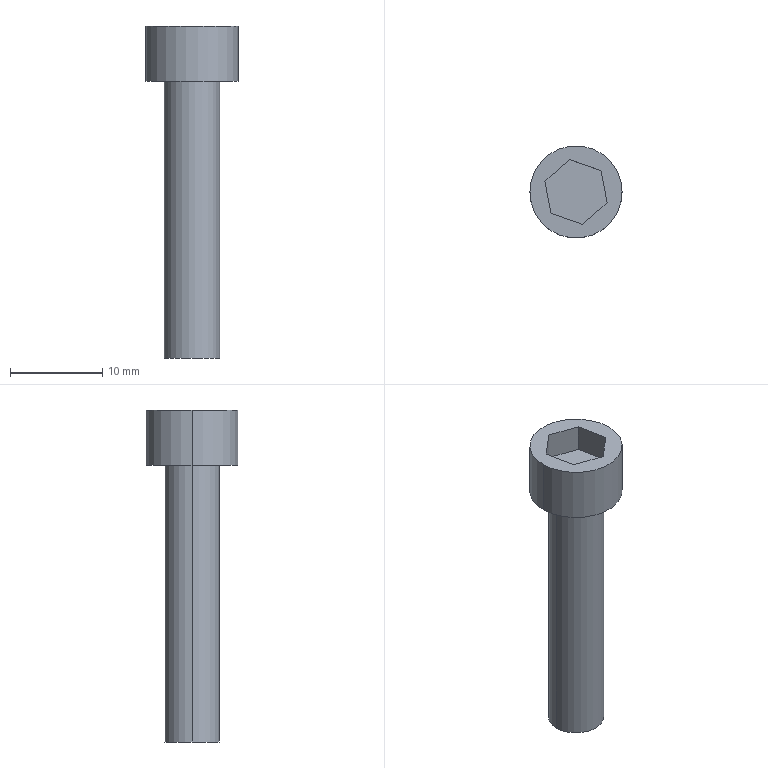Part | STEP file | M6 | 1 solid | 14 faces | box 10 x 10 x 36 mm | volume 1220 mm3 | plane 10 | cylinder 4 | commonest cylinder face diameters 6 x2 10 x2
STEP:
#1=CARTESIAN_POINT('',(0.,0.,0.));
#2=DIRECTION('',(0.,0.,1.));
#3=DIRECTION('',(1.,0.,0.));
#4=AXIS2_PLACEMENT_3D('',#1,#2,#3);
#5=CARTESIAN_POINT('',(-3.,0.,-30.));
#6=VERTEX_POINT('',#5);
#7=CARTESIAN_POINT('',(3.,0.,-30.));
#8=VERTEX_POINT('',#7);
#9=CARTESIAN_POINT('',(0.,0.,-30.));
#10=DIRECTION('',(0.,0.,-1.));
#11=DIRECTION('',(-1.,0.,0.));
#12=AXIS2_PLACEMENT_3D('',#9,#10,#11);
#13=CIRCLE('',#12,3.);
#14=CARTESIAN_POINT('',(0.,0.,-30.));
#15=DIRECTION('',(0.,0.,1.));
#16=DIRECTION('',(1.,0.,0.));
#17=AXIS2_PLACEMENT_3D('',#14,#15,#16);
#18=CYLINDRICAL_SURFACE('',#17,3.);
#19=CARTESIAN_POINT('',(3.142,0.));
#20=DIRECTION('',(-1.,0.));
#21=VECTOR('',#20,1.);
#22=LINE('',#19,#21);
#23=(GEOMETRIC_REPRESENTATION_CONTEXT(2)PARAMETRIC_REPRESENTATION_CONTEXT()REPRESENTATION_CONTEXT('',''));
#24=DEFINITIONAL_REPRESENTATION('',(#22),#23);
#25=PCURVE('',#18,#24);
#26=CARTESIAN_POINT('',(0.,0.,-30.));
#27=DIRECTION('',(0.,0.,-1.));
#28=DIRECTION('',(-1.,0.,0.));
#29=AXIS2_PLACEMENT_3D('',#26,#27,#28);
#30=PLANE('',#29);
#31=CARTESIAN_POINT('',(0.,0.));
#32=DIRECTION('',(1.,0.));
#33=AXIS2_PLACEMENT_2D('',#31,#32);
#34=CIRCLE('',#33,3.);
#35=(GEOMETRIC_REPRESENTATION_CONTEXT(2)PARAMETRIC_REPRESENTATION_CONTEXT()REPRESENTATION_CONTEXT('',''));
#36=DEFINITIONAL_REPRESENTATION('',(#34),#35);
#37=PCURVE('',#30,#36);
#38=SURFACE_CURVE('',#13,(#25,#37),.PCURVE_S1.);
#39=EDGE_CURVE('',#6,#8,#38,.T.);
#40=ORIENTED_EDGE('',*,*,#39,.F.);
#41=CARTESIAN_POINT('',(-3.,0.,0.));
#42=VERTEX_POINT('',#41);
#43=CARTESIAN_POINT('',(-3.,0.,-30.));
#44=DIRECTION('',(0.,0.,1.));
#45=VECTOR('',#44,1.);
#46=LINE('',#43,#45);
#47=CARTESIAN_POINT('',(3.142,0.));
#48=DIRECTION('',(0.,1.));
#49=VECTOR('',#48,1.);
#50=LINE('',#47,#49);
#51=(GEOMETRIC_REPRESENTATION_CONTEXT(2)PARAMETRIC_REPRESENTATION_CONTEXT()REPRESENTATION_CONTEXT('',''));
#52=DEFINITIONAL_REPRESENTATION('',(#50),#51);
#53=PCURVE('',#18,#52);
#54=CARTESIAN_POINT('',(0.,0.,-30.));
#55=DIRECTION('',(0.,0.,1.));
#56=DIRECTION('',(1.,0.,0.));
#57=AXIS2_PLACEMENT_3D('',#54,#55,#56);
#58=CYLINDRICAL_SURFACE('',#57,3.);
#59=CARTESIAN_POINT('',(3.142,0.));
#60=DIRECTION('',(0.,1.));
#61=VECTOR('',#60,1.);
#62=LINE('',#59,#61);
#63=(GEOMETRIC_REPRESENTATION_CONTEXT(2)PARAMETRIC_REPRESENTATION_CONTEXT()REPRESENTATION_CONTEXT('',''));
#64=DEFINITIONAL_REPRESENTATION('',(#62),#63);
#65=PCURVE('',#58,#64);
#66=SURFACE_CURVE('',#46,(#53,#65),.PCURVE_S1.);
#67=EDGE_CURVE('',#6,#42,#66,.T.);
#68=ORIENTED_EDGE('',*,*,#67,.T.);
#69=CARTESIAN_POINT('',(3.,0.,0.));
#70=VERTEX_POINT('',#69);
#71=CARTESIAN_POINT('',(0.,0.,0.));
#72=DIRECTION('',(0.,0.,-1.));
#73=DIRECTION('',(1.,0.,0.));
#74=AXIS2_PLACEMENT_3D('',#71,#72,#73);
#75=CIRCLE('',#74,3.);
#76=CARTESIAN_POINT('',(6.283,30.));
#77=DIRECTION('',(-1.,0.));
#78=VECTOR('',#77,1.);
#79=LINE('',#76,#78);
#80=(GEOMETRIC_REPRESENTATION_CONTEXT(2)PARAMETRIC_REPRESENTATION_CONTEXT()REPRESENTATION_CONTEXT('',''));
#81=DEFINITIONAL_REPRESENTATION('',(#79),#80);
#82=PCURVE('',#18,#81);
#83=CARTESIAN_POINT('',(0.,0.,0.));
#84=DIRECTION('',(0.,0.,1.));
#85=DIRECTION('',(1.,0.,0.));
#86=AXIS2_PLACEMENT_3D('',#83,#84,#85);
#87=PLANE('',#86);
#88=CARTESIAN_POINT('',(3.,0.));
#89=CARTESIAN_POINT('',(3.,-5.196));
#90=CARTESIAN_POINT('',(-1.5,-2.598));
#91=CARTESIAN_POINT('',(-6.,0.));
#92=CARTESIAN_POINT('',(-1.5,2.598));
#93=CARTESIAN_POINT('',(3.,5.196));
#94=CARTESIAN_POINT('',(3.,0.));
#95=(BOUNDED_CURVE()B_SPLINE_CURVE(2,(#88,#89,#90,#91,#92,#93,#94),.UNSPECIFIED.,.T.,.F.)B_SPLINE_CURVE_WITH_KNOTS((1,2,2,2,2,1),(-2.094,0.,2.094,4.189,6.283,8.378),.UNSPECIFIED.)CURVE()GEOMETRIC_REPRESENTATION_ITEM()RATIONAL_B_SPLINE_CURVE((1.,0.5,1.,0.5,1.,0.5,1.))REPRESENTATION_ITEM(''));
#96=(GEOMETRIC_REPRESENTATION_CONTEXT(2)PARAMETRIC_REPRESENTATION_CONTEXT()REPRESENTATION_CONTEXT('',''));
#97=DEFINITIONAL_REPRESENTATION('',(#95),#96);
#98=PCURVE('',#87,#97);
#99=SURFACE_CURVE('',#75,(#82,#98),.PCURVE_S1.);
#100=EDGE_CURVE('',#42,#70,#99,.T.);
#101=ORIENTED_EDGE('',*,*,#100,.T.);
#102=CARTESIAN_POINT('',(3.,0.,-30.));
#103=DIRECTION('',(0.,0.,1.));
#104=VECTOR('',#103,1.);
#105=LINE('',#102,#104);
#106=CARTESIAN_POINT('',(0.,0.));
#107=DIRECTION('',(0.,1.));
#108=VECTOR('',#107,1.);
#109=LINE('',#106,#108);
#110=(GEOMETRIC_REPRESENTATION_CONTEXT(2)PARAMETRIC_REPRESENTATION_CONTEXT()REPRESENTATION_CONTEXT('',''));
#111=DEFINITIONAL_REPRESENTATION('',(#109),#110);
#112=PCURVE('',#18,#111);
#113=CARTESIAN_POINT('',(6.283,0.));
#114=DIRECTION('',(0.,1.));
#115=VECTOR('',#114,1.);
#116=LINE('',#113,#115);
#117=(GEOMETRIC_REPRESENTATION_CONTEXT(2)PARAMETRIC_REPRESENTATION_CONTEXT()REPRESENTATION_CONTEXT('',''));
#118=DEFINITIONAL_REPRESENTATION('',(#116),#117);
#119=PCURVE('',#58,#118);
#120=SURFACE_CURVE('',#105,(#112,#119),.PCURVE_S1.);
#121=EDGE_CURVE('',#8,#70,#120,.T.);
#122=ORIENTED_EDGE('',*,*,#121,.F.);
#123=EDGE_LOOP('',(#40,#68,#101,#122));
#124=FACE_BOUND('',#123,.T.);
#125=ADVANCED_FACE('',(#124),#18,.T.);
#126=CARTESIAN_POINT('',(5.,0.,6.));
#127=VERTEX_POINT('',#126);
#128=CARTESIAN_POINT('',(-5.,0.,6.));
#129=VERTEX_POINT('',#128);
#130=CARTESIAN_POINT('',(0.,0.,6.));
#131=DIRECTION('',(0.,0.,1.));
#132=DIRECTION('',(1.,0.,0.));
#133=AXIS2_PLACEMENT_3D('',#130,#131,#132);
#134=CIRCLE('',#133,5.);
#135=CARTESIAN_POINT('',(0.,0.,6.));
#136=DIRECTION('',(0.,0.,-1.));
#137=DIRECTION('',(-1.,0.,0.));
#138=AXIS2_PLACEMENT_3D('',#135,#136,#137);
#139=CYLINDRICAL_SURFACE('',#138,5.);
#140=CARTESIAN_POINT('',(3.142,0.));
#141=DIRECTION('',(-1.,0.));
#142=VECTOR('',#141,1.);
#143=LINE('',#140,#142);
#144=(GEOMETRIC_REPRESENTATION_CONTEXT(2)PARAMETRIC_REPRESENTATION_CONTEXT()REPRESENTATION_CONTEXT('',''));
#145=DEFINITIONAL_REPRESENTATION('',(#143),#144);
#146=PCURVE('',#139,#145);
#147=CARTESIAN_POINT('',(0.,0.,6.));
#148=DIRECTION('',(0.,0.,1.));
#149=DIRECTION('',(1.,0.,0.));
#150=AXIS2_PLACEMENT_3D('',#147,#148,#149);
#151=PLANE('',#150);
#152=CARTESIAN_POINT('',(0.,0.));
#153=DIRECTION('',(1.,0.));
#154=AXIS2_PLACEMENT_2D('',#152,#153);
#155=CIRCLE('',#154,5.);
#156=(GEOMETRIC_REPRESENTATION_CONTEXT(2)PARAMETRIC_REPRESENTATION_CONTEXT()REPRESENTATION_CONTEXT('',''));
#157=DEFINITIONAL_REPRESENTATION('',(#155),#156);
#158=PCURVE('',#151,#157);
#159=SURFACE_CURVE('',#134,(#146,#158),.PCURVE_S1.);
#160=EDGE_CURVE('',#127,#129,#159,.T.);
#161=ORIENTED_EDGE('',*,*,#160,.F.);
#162=CARTESIAN_POINT('',(5.,0.,0.));
#163=VERTEX_POINT('',#162);
#164=CARTESIAN_POINT('',(5.,0.,6.));
#165=DIRECTION('',(0.,0.,-1.));
#166=VECTOR('',#165,1.);
#167=LINE('',#164,#166);
#168=CARTESIAN_POINT('',(3.142,0.));
#169=DIRECTION('',(0.,1.));
#170=VECTOR('',#169,1.);
#171=LINE('',#168,#170);
#172=(GEOMETRIC_REPRESENTATION_CONTEXT(2)PARAMETRIC_REPRESENTATION_CONTEXT()REPRESENTATION_CONTEXT('',''));
#173=DEFINITIONAL_REPRESENTATION('',(#171),#172);
#174=PCURVE('',#139,#173);
#175=CARTESIAN_POINT('',(0.,0.,6.));
#176=DIRECTION('',(0.,0.,-1.));
#177=DIRECTION('',(-1.,0.,0.));
#178=AXIS2_PLACEMENT_3D('',#175,#176,#177);
#179=CYLINDRICAL_SURFACE('',#178,5.);
#180=CARTESIAN_POINT('',(3.142,0.));
#181=DIRECTION('',(0.,1.));
#182=VECTOR('',#181,1.);
#183=LINE('',#180,#182);
#184=(GEOMETRIC_REPRESENTATION_CONTEXT(2)PARAMETRIC_REPRESENTATION_CONTEXT()REPRESENTATION_CONTEXT('',''));
#185=DEFINITIONAL_REPRESENTATION('',(#183),#184);
#186=PCURVE('',#179,#185);
#187=SURFACE_CURVE('',#167,(#174,#186),.PCURVE_S1.);
#188=EDGE_CURVE('',#127,#163,#187,.T.);
#189=ORIENTED_EDGE('',*,*,#188,.T.);
#190=CARTESIAN_POINT('',(-5.,0.,0.));
#191=VERTEX_POINT('',#190);
#192=CARTESIAN_POINT('',(0.,0.,0.));
#193=DIRECTION('',(0.,0.,1.));
#194=DIRECTION('',(1.,0.,0.));
#195=AXIS2_PLACEMENT_3D('',#192,#193,#194);
#196=CIRCLE('',#195,5.);
#197=CARTESIAN_POINT('',(3.142,6.));
#198=DIRECTION('',(-1.,0.));
#199=VECTOR('',#198,1.);
#200=LINE('',#197,#199);
#201=(GEOMETRIC_REPRESENTATION_CONTEXT(2)PARAMETRIC_REPRESENTATION_CONTEXT()REPRESENTATION_CONTEXT('',''));
#202=DEFINITIONAL_REPRESENTATION('',(#200),#201);
#203=PCURVE('',#139,#202);
#204=CARTESIAN_POINT('',(0.,0.));
#205=DIRECTION('',(1.,0.));
#206=AXIS2_PLACEMENT_2D('',#204,#205);
#207=CIRCLE('',#206,5.);
#208=(GEOMETRIC_REPRESENTATION_CONTEXT(2)PARAMETRIC_REPRESENTATION_CONTEXT()REPRESENTATION_CONTEXT('',''));
#209=DEFINITIONAL_REPRESENTATION('',(#207),#208);
#210=PCURVE('',#87,#209);
#211=SURFACE_CURVE('',#196,(#203,#210),.PCURVE_S1.);
#212=EDGE_CURVE('',#163,#191,#211,.T.);
#213=ORIENTED_EDGE('',*,*,#212,.T.);
#214=CARTESIAN_POINT('',(-5.,0.,6.));
#215=DIRECTION('',(0.,0.,-1.));
#216=VECTOR('',#215,1.);
#217=LINE('',#214,#216);
#218=CARTESIAN_POINT('',(0.,0.));
#219=DIRECTION('',(0.,1.));
#220=VECTOR('',#219,1.);
#221=LINE('',#218,#220);
#222=(GEOMETRIC_REPRESENTATION_CONTEXT(2)PARAMETRIC_REPRESENTATION_CONTEXT()REPRESENTATION_CONTEXT('',''));
#223=DEFINITIONAL_REPRESENTATION('',(#221),#222);
#224=PCURVE('',#139,#223);
#225=CARTESIAN_POINT('',(6.283,0.));
#226=DIRECTION('',(0.,1.));
#227=VECTOR('',#226,1.);
#228=LINE('',#225,#227);
#229=(GEOMETRIC_REPRESENTATION_CONTEXT(2)PARAMETRIC_REPRESENTATION_CONTEXT()REPRESENTATION_CONTEXT('',''));
#230=DEFINITIONAL_REPRESENTATION('',(#228),#229);
#231=PCURVE('',#179,#230);
#232=SURFACE_CURVE('',#217,(#224,#231),.PCURVE_S1.);
#233=EDGE_CURVE('',#129,#191,#232,.T.);
#234=ORIENTED_EDGE('',*,*,#233,.F.);
#235=EDGE_LOOP('',(#161,#189,#213,#234));
#236=FACE_BOUND('',#235,.T.);
#237=ADVANCED_FACE('',(#236),#139,.T.);
#238=CARTESIAN_POINT('',(0.,0.,0.));
#239=DIRECTION('',(0.,0.,1.));
#240=DIRECTION('',(1.,0.,0.));
#241=AXIS2_PLACEMENT_3D('',#238,#239,#240);
#242=CIRCLE('',#241,5.);
#243=CARTESIAN_POINT('',(0.,0.));
#244=DIRECTION('',(1.,0.));
#245=AXIS2_PLACEMENT_2D('',#243,#244);
#246=CIRCLE('',#245,5.);
#247=(GEOMETRIC_REPRESENTATION_CONTEXT(2)PARAMETRIC_REPRESENTATION_CONTEXT()REPRESENTATION_CONTEXT('',''));
#248=DEFINITIONAL_REPRESENTATION('',(#246),#247);
#249=PCURVE('',#87,#248);
#250=CARTESIAN_POINT('',(9.425,6.));
#251=DIRECTION('',(-1.,0.));
#252=VECTOR('',#251,1.);
#253=LINE('',#250,#252);
#254=(GEOMETRIC_REPRESENTATION_CONTEXT(2)PARAMETRIC_REPRESENTATION_CONTEXT()REPRESENTATION_CONTEXT('',''));
#255=DEFINITIONAL_REPRESENTATION('',(#253),#254);
#256=PCURVE('',#179,#255);
#257=SURFACE_CURVE('',#242,(#249,#256),.PCURVE_S1.);
#258=EDGE_CURVE('',#191,#163,#257,.T.);
#259=ORIENTED_EDGE('',*,*,#258,.F.);
#260=ORIENTED_EDGE('',*,*,#212,.F.);
#261=EDGE_LOOP('',(#259,#260));
#262=FACE_BOUND('',#261,.T.);
#263=CARTESIAN_POINT('',(0.,0.,0.));
#264=DIRECTION('',(0.,0.,-1.));
#265=DIRECTION('',(1.,0.,0.));
#266=AXIS2_PLACEMENT_3D('',#263,#264,#265);
#267=CIRCLE('',#266,3.);
#268=CARTESIAN_POINT('',(3.,0.));
#269=CARTESIAN_POINT('',(3.,-5.196));
#270=CARTESIAN_POINT('',(-1.5,-2.598));
#271=CARTESIAN_POINT('',(-6.,0.));
#272=CARTESIAN_POINT('',(-1.5,2.598));
#273=CARTESIAN_POINT('',(3.,5.196));
#274=CARTESIAN_POINT('',(3.,0.));
#275=(BOUNDED_CURVE()B_SPLINE_CURVE(2,(#268,#269,#270,#271,#272,#273,#274),.UNSPECIFIED.,.T.,.F.)B_SPLINE_CURVE_WITH_KNOTS((1,2,2,2,2,1),(-2.094,0.,2.094,4.189,6.283,8.378),.UNSPECIFIED.)CURVE()GEOMETRIC_REPRESENTATION_ITEM()RATIONAL_B_SPLINE_CURVE((1.,0.5,1.,0.5,1.,0.5,1.))REPRESENTATION_ITEM(''));
#276=(GEOMETRIC_REPRESENTATION_CONTEXT(2)PARAMETRIC_REPRESENTATION_CONTEXT()REPRESENTATION_CONTEXT('',''));
#277=DEFINITIONAL_REPRESENTATION('',(#275),#276);
#278=PCURVE('',#87,#277);
#279=CARTESIAN_POINT('',(6.283,30.));
#280=DIRECTION('',(-1.,0.));
#281=VECTOR('',#280,1.);
#282=LINE('',#279,#281);
#283=(GEOMETRIC_REPRESENTATION_CONTEXT(2)PARAMETRIC_REPRESENTATION_CONTEXT()REPRESENTATION_CONTEXT('',''));
#284=DEFINITIONAL_REPRESENTATION('',(#282),#283);
#285=PCURVE('',#58,#284);
#286=SURFACE_CURVE('',#267,(#278,#285),.PCURVE_S1.);
#287=EDGE_CURVE('',#70,#42,#286,.T.);
#288=ORIENTED_EDGE('',*,*,#287,.F.);
#289=ORIENTED_EDGE('',*,*,#100,.F.);
#290=EDGE_LOOP('',(#288,#289));
#291=FACE_BOUND('',#290,.T.);
#292=ADVANCED_FACE('',(#262,#291),#87,.F.);
#293=ORIENTED_EDGE('',*,*,#188,.F.);
#294=CARTESIAN_POINT('',(0.,0.,6.));
#295=DIRECTION('',(0.,0.,1.));
#296=DIRECTION('',(1.,0.,0.));
#297=AXIS2_PLACEMENT_3D('',#294,#295,#296);
#298=CIRCLE('',#297,5.);
#299=CARTESIAN_POINT('',(9.425,0.));
#300=DIRECTION('',(-1.,0.));
#301=VECTOR('',#300,1.);
#302=LINE('',#299,#301);
#303=(GEOMETRIC_REPRESENTATION_CONTEXT(2)PARAMETRIC_REPRESENTATION_CONTEXT()REPRESENTATION_CONTEXT('',''));
#304=DEFINITIONAL_REPRESENTATION('',(#302),#303);
#305=PCURVE('',#179,#304);
#306=CARTESIAN_POINT('',(0.,0.));
#307=DIRECTION('',(1.,0.));
#308=AXIS2_PLACEMENT_2D('',#306,#307);
#309=CIRCLE('',#308,5.);
#310=(GEOMETRIC_REPRESENTATION_CONTEXT(2)PARAMETRIC_REPRESENTATION_CONTEXT()REPRESENTATION_CONTEXT('',''));
#311=DEFINITIONAL_REPRESENTATION('',(#309),#310);
#312=PCURVE('',#151,#311);
#313=SURFACE_CURVE('',#298,(#305,#312),.PCURVE_S1.);
#314=EDGE_CURVE('',#129,#127,#313,.T.);
#315=ORIENTED_EDGE('',*,*,#314,.F.);
#316=ORIENTED_EDGE('',*,*,#233,.T.);
#317=ORIENTED_EDGE('',*,*,#258,.T.);
#318=EDGE_LOOP('',(#293,#315,#316,#317));
#319=FACE_BOUND('',#318,.T.);
#320=ADVANCED_FACE('',(#319),#179,.T.);
#321=CARTESIAN_POINT('',(-3.378,1.179,6.));
#322=VERTEX_POINT('',#321);
#323=CARTESIAN_POINT('',(-2.71,-2.336,6.));
#324=VERTEX_POINT('',#323);
#325=CARTESIAN_POINT('',(-3.378,1.179,6.));
#326=DIRECTION('',(0.1867,-0.9824,0.));
#327=VECTOR('',#326,1.);
#328=LINE('',#325,#327);
#329=CARTESIAN_POINT('',(-3.378,1.179));
#330=DIRECTION('',(0.1867,-0.9824));
#331=VECTOR('',#330,1.);
#332=LINE('',#329,#331);
#333=(GEOMETRIC_REPRESENTATION_CONTEXT(2)PARAMETRIC_REPRESENTATION_CONTEXT()REPRESENTATION_CONTEXT('',''));
#334=DEFINITIONAL_REPRESENTATION('',(#332),#333);
#335=PCURVE('',#151,#334);
#336=CARTESIAN_POINT('',(-3.378,1.179,3.));
#337=DIRECTION('',(-0.9824,-0.1867,0.));
#338=DIRECTION('',(0.1867,-0.9824,0.));
#339=AXIS2_PLACEMENT_3D('',#336,#337,#338);
#340=PLANE('',#339);
#341=CARTESIAN_POINT('',(0.,3.));
#342=DIRECTION('',(1.,0.));
#343=VECTOR('',#342,1.);
#344=LINE('',#341,#343);
#345=(GEOMETRIC_REPRESENTATION_CONTEXT(2)PARAMETRIC_REPRESENTATION_CONTEXT()REPRESENTATION_CONTEXT('',''));
#346=DEFINITIONAL_REPRESENTATION('',(#344),#345);
#347=PCURVE('',#340,#346);
#348=SURFACE_CURVE('',#328,(#335,#347),.PCURVE_S1.);
#349=EDGE_CURVE('',#322,#324,#348,.T.);
#350=ORIENTED_EDGE('',*,*,#349,.F.);
#351=CARTESIAN_POINT('',(-0.6678,3.514,6.));
#352=VERTEX_POINT('',#351);
#353=CARTESIAN_POINT('',(-0.6678,3.514,6.));
#354=DIRECTION('',(-0.7575,-0.6529,0.));
#355=VECTOR('',#354,1.);
#356=LINE('',#353,#355);
#357=CARTESIAN_POINT('',(-0.6678,3.514));
#358=DIRECTION('',(-0.7575,-0.6529));
#359=VECTOR('',#358,1.);
#360=LINE('',#357,#359);
#361=(GEOMETRIC_REPRESENTATION_CONTEXT(2)PARAMETRIC_REPRESENTATION_CONTEXT()REPRESENTATION_CONTEXT('',''));
#362=DEFINITIONAL_REPRESENTATION('',(#360),#361);
#363=PCURVE('',#151,#362);
#364=CARTESIAN_POINT('',(-0.6678,3.514,3.));
#365=DIRECTION('',(-0.6529,0.7575,0.));
#366=DIRECTION('',(-0.7575,-0.6529,0.));
#367=AXIS2_PLACEMENT_3D('',#364,#365,#366);
#368=PLANE('',#367);
#369=CARTESIAN_POINT('',(0.,3.));
#370=DIRECTION('',(1.,0.));
#371=VECTOR('',#370,1.);
#372=LINE('',#369,#371);
#373=(GEOMETRIC_REPRESENTATION_CONTEXT(2)PARAMETRIC_REPRESENTATION_CONTEXT()REPRESENTATION_CONTEXT('',''));
#374=DEFINITIONAL_REPRESENTATION('',(#372),#373);
#375=PCURVE('',#368,#374);
#376=SURFACE_CURVE('',#356,(#363,#375),.PCURVE_S1.);
#377=EDGE_CURVE('',#352,#322,#376,.T.);
#378=ORIENTED_EDGE('',*,*,#377,.F.);
#379=CARTESIAN_POINT('',(2.71,2.336,6.));
#380=VERTEX_POINT('',#379);
#381=CARTESIAN_POINT('',(2.71,2.336,6.));
#382=DIRECTION('',(-0.9441,0.3295,0.));
#383=VECTOR('',#382,1.);
#384=LINE('',#381,#383);
#385=CARTESIAN_POINT('',(2.71,2.336));
#386=DIRECTION('',(-0.9441,0.3295));
#387=VECTOR('',#386,1.);
#388=LINE('',#385,#387);
#389=(GEOMETRIC_REPRESENTATION_CONTEXT(2)PARAMETRIC_REPRESENTATION_CONTEXT()REPRESENTATION_CONTEXT('',''));
#390=DEFINITIONAL_REPRESENTATION('',(#388),#389);
#391=PCURVE('',#151,#390);
#392=CARTESIAN_POINT('',(2.71,2.336,3.));
#393=DIRECTION('',(0.3295,0.9441,0.));
#394=DIRECTION('',(-0.9441,0.3295,0.));
#395=AXIS2_PLACEMENT_3D('',#392,#393,#394);
#396=PLANE('',#395);
#397=CARTESIAN_POINT('',(0.,3.));
#398=DIRECTION('',(1.,0.));
#399=VECTOR('',#398,1.);
#400=LINE('',#397,#399);
#401=(GEOMETRIC_REPRESENTATION_CONTEXT(2)PARAMETRIC_REPRESENTATION_CONTEXT()REPRESENTATION_CONTEXT('',''));
#402=DEFINITIONAL_REPRESENTATION('',(#400),#401);
#403=PCURVE('',#396,#402);
#404=SURFACE_CURVE('',#384,(#391,#403),.PCURVE_S1.);
#405=EDGE_CURVE('',#380,#352,#404,.T.);
#406=ORIENTED_EDGE('',*,*,#405,.F.);
#407=CARTESIAN_POINT('',(3.378,-1.179,6.));
#408=VERTEX_POINT('',#407);
#409=CARTESIAN_POINT('',(3.378,-1.179,6.));
#410=DIRECTION('',(-0.1867,0.9824,0.));
#411=VECTOR('',#410,1.);
#412=LINE('',#409,#411);
#413=CARTESIAN_POINT('',(3.378,-1.179));
#414=DIRECTION('',(-0.1867,0.9824));
#415=VECTOR('',#414,1.);
#416=LINE('',#413,#415);
#417=(GEOMETRIC_REPRESENTATION_CONTEXT(2)PARAMETRIC_REPRESENTATION_CONTEXT()REPRESENTATION_CONTEXT('',''));
#418=DEFINITIONAL_REPRESENTATION('',(#416),#417);
#419=PCURVE('',#151,#418);
#420=CARTESIAN_POINT('',(3.378,-1.179,3.));
#421=DIRECTION('',(0.9824,0.1867,0.));
#422=DIRECTION('',(-0.1867,0.9824,0.));
#423=AXIS2_PLACEMENT_3D('',#420,#421,#422);
#424=PLANE('',#423);
#425=CARTESIAN_POINT('',(0.,3.));
#426=DIRECTION('',(1.,0.));
#427=VECTOR('',#426,1.);
#428=LINE('',#425,#427);
#429=(GEOMETRIC_REPRESENTATION_CONTEXT(2)PARAMETRIC_REPRESENTATION_CONTEXT()REPRESENTATION_CONTEXT('',''));
#430=DEFINITIONAL_REPRESENTATION('',(#428),#429);
#431=PCURVE('',#424,#430);
#432=SURFACE_CURVE('',#412,(#419,#431),.PCURVE_S1.);
#433=EDGE_CURVE('',#408,#380,#432,.T.);
#434=ORIENTED_EDGE('',*,*,#433,.F.);
#435=CARTESIAN_POINT('',(0.6678,-3.514,6.));
#436=VERTEX_POINT('',#435);
#437=CARTESIAN_POINT('',(0.6678,-3.514,6.));
#438=DIRECTION('',(0.7575,0.6529,0.));
#439=VECTOR('',#438,1.);
#440=LINE('',#437,#439);
#441=CARTESIAN_POINT('',(0.6678,-3.514));
#442=DIRECTION('',(0.7575,0.6529));
#443=VECTOR('',#442,1.);
#444=LINE('',#441,#443);
#445=(GEOMETRIC_REPRESENTATION_CONTEXT(2)PARAMETRIC_REPRESENTATION_CONTEXT()REPRESENTATION_CONTEXT('',''));
#446=DEFINITIONAL_REPRESENTATION('',(#444),#445);
#447=PCURVE('',#151,#446);
#448=CARTESIAN_POINT('',(0.6678,-3.514,3.));
#449=DIRECTION('',(0.6529,-0.7575,0.));
#450=DIRECTION('',(0.7575,0.6529,0.));
#451=AXIS2_PLACEMENT_3D('',#448,#449,#450);
#452=PLANE('',#451);
#453=CARTESIAN_POINT('',(0.,3.));
#454=DIRECTION('',(1.,0.));
#455=VECTOR('',#454,1.);
#456=LINE('',#453,#455);
#457=(GEOMETRIC_REPRESENTATION_CONTEXT(2)PARAMETRIC_REPRESENTATION_CONTEXT()REPRESENTATION_CONTEXT('',''));
#458=DEFINITIONAL_REPRESENTATION('',(#456),#457);
#459=PCURVE('',#452,#458);
#460=SURFACE_CURVE('',#440,(#447,#459),.PCURVE_S1.);
#461=EDGE_CURVE('',#436,#408,#460,.T.);
#462=ORIENTED_EDGE('',*,*,#461,.F.);
#463=CARTESIAN_POINT('',(-2.71,-2.336,6.));
#464=DIRECTION('',(0.9441,-0.3295,0.));
#465=VECTOR('',#464,1.);
#466=LINE('',#463,#465);
#467=CARTESIAN_POINT('',(-2.71,-2.336));
#468=DIRECTION('',(0.9441,-0.3295));
#469=VECTOR('',#468,1.);
#470=LINE('',#467,#469);
#471=(GEOMETRIC_REPRESENTATION_CONTEXT(2)PARAMETRIC_REPRESENTATION_CONTEXT()REPRESENTATION_CONTEXT('',''));
#472=DEFINITIONAL_REPRESENTATION('',(#470),#471);
#473=PCURVE('',#151,#472);
#474=CARTESIAN_POINT('',(-2.71,-2.336,3.));
#475=DIRECTION('',(-0.3295,-0.9441,0.));
#476=DIRECTION('',(0.9441,-0.3295,0.));
#477=AXIS2_PLACEMENT_3D('',#474,#475,#476);
#478=PLANE('',#477);
#479=CARTESIAN_POINT('',(0.,3.));
#480=DIRECTION('',(1.,0.));
#481=VECTOR('',#480,1.);
#482=LINE('',#479,#481);
#483=(GEOMETRIC_REPRESENTATION_CONTEXT(2)PARAMETRIC_REPRESENTATION_CONTEXT()REPRESENTATION_CONTEXT('',''));
#484=DEFINITIONAL_REPRESENTATION('',(#482),#483);
#485=PCURVE('',#478,#484);
#486=SURFACE_CURVE('',#466,(#473,#485),.PCURVE_S1.);
#487=EDGE_CURVE('',#324,#436,#486,.T.);
#488=ORIENTED_EDGE('',*,*,#487,.F.);
#489=EDGE_LOOP('',(#350,#378,#406,#434,#462,#488));
#490=FACE_BOUND('',#489,.T.);
#491=ORIENTED_EDGE('',*,*,#314,.T.);
#492=ORIENTED_EDGE('',*,*,#160,.T.);
#493=EDGE_LOOP('',(#491,#492));
#494=FACE_BOUND('',#493,.T.);
#495=ADVANCED_FACE('',(#490,#494),#151,.T.);
#496=ORIENTED_EDGE('',*,*,#67,.F.);
#497=CARTESIAN_POINT('',(0.,0.,-30.));
#498=DIRECTION('',(0.,0.,-1.));
#499=DIRECTION('',(-1.,0.,0.));
#500=AXIS2_PLACEMENT_3D('',#497,#498,#499);
#501=CIRCLE('',#500,3.);
#502=CARTESIAN_POINT('',(9.425,0.));
#503=DIRECTION('',(-1.,0.));
#504=VECTOR('',#503,1.);
#505=LINE('',#502,#504);
#506=(GEOMETRIC_REPRESENTATION_CONTEXT(2)PARAMETRIC_REPRESENTATION_CONTEXT()REPRESENTATION_CONTEXT('',''));
#507=DEFINITIONAL_REPRESENTATION('',(#505),#506);
#508=PCURVE('',#58,#507);
#509=CARTESIAN_POINT('',(0.,0.));
#510=DIRECTION('',(1.,0.));
#511=AXIS2_PLACEMENT_2D('',#509,#510);
#512=CIRCLE('',#511,3.);
#513=(GEOMETRIC_REPRESENTATION_CONTEXT(2)PARAMETRIC_REPRESENTATION_CONTEXT()REPRESENTATION_CONTEXT('',''));
#514=DEFINITIONAL_REPRESENTATION('',(#512),#513);
#515=PCURVE('',#30,#514);
#516=SURFACE_CURVE('',#501,(#508,#515),.PCURVE_S1.);
#517=EDGE_CURVE('',#8,#6,#516,.T.);
#518=ORIENTED_EDGE('',*,*,#517,.F.);
#519=ORIENTED_EDGE('',*,*,#121,.T.);
#520=ORIENTED_EDGE('',*,*,#287,.T.);
#521=EDGE_LOOP('',(#496,#518,#519,#520));
#522=FACE_BOUND('',#521,.T.);
#523=ADVANCED_FACE('',(#522),#58,.T.);
#524=ORIENTED_EDGE('',*,*,#517,.T.);
#525=ORIENTED_EDGE('',*,*,#39,.T.);
#526=EDGE_LOOP('',(#524,#525));
#527=FACE_BOUND('',#526,.T.);
#528=ADVANCED_FACE('',(#527),#30,.T.);
#529=ORIENTED_EDGE('',*,*,#349,.T.);
#530=CARTESIAN_POINT('',(-2.71,-2.336,3.));
#531=VERTEX_POINT('',#530);
#532=CARTESIAN_POINT('',(-2.71,-2.336,3.));
#533=DIRECTION('',(0.,0.,1.));
#534=VECTOR('',#533,1.);
#535=LINE('',#532,#534);
#536=CARTESIAN_POINT('',(3.577,0.));
#537=DIRECTION('',(0.,1.));
#538=VECTOR('',#537,1.);
#539=LINE('',#536,#538);
#540=(GEOMETRIC_REPRESENTATION_CONTEXT(2)PARAMETRIC_REPRESENTATION_CONTEXT()REPRESENTATION_CONTEXT('',''));
#541=DEFINITIONAL_REPRESENTATION('',(#539),#540);
#542=PCURVE('',#340,#541);
#543=CARTESIAN_POINT('',(0.,0.));
#544=DIRECTION('',(0.,1.));
#545=VECTOR('',#544,1.);
#546=LINE('',#543,#545);
#547=(GEOMETRIC_REPRESENTATION_CONTEXT(2)PARAMETRIC_REPRESENTATION_CONTEXT()REPRESENTATION_CONTEXT('',''));
#548=DEFINITIONAL_REPRESENTATION('',(#546),#547);
#549=PCURVE('',#478,#548);
#550=SURFACE_CURVE('',#535,(#542,#549),.PCURVE_S1.);
#551=EDGE_CURVE('',#531,#324,#550,.T.);
#552=ORIENTED_EDGE('',*,*,#551,.F.);
#553=CARTESIAN_POINT('',(-3.378,1.179,3.));
#554=VERTEX_POINT('',#553);
#555=CARTESIAN_POINT('',(-3.378,1.179,3.));
#556=DIRECTION('',(0.1867,-0.9824,0.));
#557=VECTOR('',#556,1.);
#558=LINE('',#555,#557);
#559=CARTESIAN_POINT('',(0.,0.));
#560=DIRECTION('',(1.,0.));
#561=VECTOR('',#560,1.);
#562=LINE('',#559,#561);
#563=(GEOMETRIC_REPRESENTATION_CONTEXT(2)PARAMETRIC_REPRESENTATION_CONTEXT()REPRESENTATION_CONTEXT('',''));
#564=DEFINITIONAL_REPRESENTATION('',(#562),#563);
#565=PCURVE('',#340,#564);
#566=CARTESIAN_POINT('',(0.,0.,3.));
#567=DIRECTION('',(0.,0.,1.));
#568=DIRECTION('',(1.,0.,0.));
#569=AXIS2_PLACEMENT_3D('',#566,#567,#568);
#570=PLANE('',#569);
#571=CARTESIAN_POINT('',(-3.378,1.179));
#572=DIRECTION('',(0.1867,-0.9824));
#573=VECTOR('',#572,1.);
#574=LINE('',#571,#573);
#575=(GEOMETRIC_REPRESENTATION_CONTEXT(2)PARAMETRIC_REPRESENTATION_CONTEXT()REPRESENTATION_CONTEXT('',''));
#576=DEFINITIONAL_REPRESENTATION('',(#574),#575);
#577=PCURVE('',#570,#576);
#578=SURFACE_CURVE('',#558,(#565,#577),.PCURVE_S1.);
#579=EDGE_CURVE('',#554,#531,#578,.T.);
#580=ORIENTED_EDGE('',*,*,#579,.F.);
#581=CARTESIAN_POINT('',(-3.378,1.179,3.));
#582=DIRECTION('',(0.,0.,1.));
#583=VECTOR('',#582,1.);
#584=LINE('',#581,#583);
#585=CARTESIAN_POINT('',(0.,0.));
#586=DIRECTION('',(0.,1.));
#587=VECTOR('',#586,1.);
#588=LINE('',#585,#587);
#589=(GEOMETRIC_REPRESENTATION_CONTEXT(2)PARAMETRIC_REPRESENTATION_CONTEXT()REPRESENTATION_CONTEXT('',''));
#590=DEFINITIONAL_REPRESENTATION('',(#588),#589);
#591=PCURVE('',#340,#590);
#592=CARTESIAN_POINT('',(3.577,0.));
#593=DIRECTION('',(0.,1.));
#594=VECTOR('',#593,1.);
#595=LINE('',#592,#594);
#596=(GEOMETRIC_REPRESENTATION_CONTEXT(2)PARAMETRIC_REPRESENTATION_CONTEXT()REPRESENTATION_CONTEXT('',''));
#597=DEFINITIONAL_REPRESENTATION('',(#595),#596);
#598=PCURVE('',#368,#597);
#599=SURFACE_CURVE('',#584,(#591,#598),.PCURVE_S1.);
#600=EDGE_CURVE('',#554,#322,#599,.T.);
#601=ORIENTED_EDGE('',*,*,#600,.T.);
#602=EDGE_LOOP('',(#529,#552,#580,#601));
#603=FACE_BOUND('',#602,.T.);
#604=ADVANCED_FACE('',(#603),#340,.F.);
#605=ORIENTED_EDGE('',*,*,#377,.T.);
#606=ORIENTED_EDGE('',*,*,#600,.F.);
#607=CARTESIAN_POINT('',(-0.6678,3.514,3.));
#608=VERTEX_POINT('',#607);
#609=CARTESIAN_POINT('',(-0.6678,3.514,3.));
#610=DIRECTION('',(-0.7575,-0.6529,0.));
#611=VECTOR('',#610,1.);
#612=LINE('',#609,#611);
#613=CARTESIAN_POINT('',(0.,0.));
#614=DIRECTION('',(1.,0.));
#615=VECTOR('',#614,1.);
#616=LINE('',#613,#615);
#617=(GEOMETRIC_REPRESENTATION_CONTEXT(2)PARAMETRIC_REPRESENTATION_CONTEXT()REPRESENTATION_CONTEXT('',''));
#618=DEFINITIONAL_REPRESENTATION('',(#616),#617);
#619=PCURVE('',#368,#618);
#620=CARTESIAN_POINT('',(-0.6678,3.514));
#621=DIRECTION('',(-0.7575,-0.6529));
#622=VECTOR('',#621,1.);
#623=LINE('',#620,#622);
#624=(GEOMETRIC_REPRESENTATION_CONTEXT(2)PARAMETRIC_REPRESENTATION_CONTEXT()REPRESENTATION_CONTEXT('',''));
#625=DEFINITIONAL_REPRESENTATION('',(#623),#624);
#626=PCURVE('',#570,#625);
#627=SURFACE_CURVE('',#612,(#619,#626),.PCURVE_S1.);
#628=EDGE_CURVE('',#608,#554,#627,.T.);
#629=ORIENTED_EDGE('',*,*,#628,.F.);
#630=CARTESIAN_POINT('',(-0.6678,3.514,3.));
#631=DIRECTION('',(0.,0.,1.));
#632=VECTOR('',#631,1.);
#633=LINE('',#630,#632);
#634=CARTESIAN_POINT('',(0.,0.));
#635=DIRECTION('',(0.,1.));
#636=VECTOR('',#635,1.);
#637=LINE('',#634,#636);
#638=(GEOMETRIC_REPRESENTATION_CONTEXT(2)PARAMETRIC_REPRESENTATION_CONTEXT()REPRESENTATION_CONTEXT('',''));
#639=DEFINITIONAL_REPRESENTATION('',(#637),#638);
#640=PCURVE('',#368,#639);
#641=CARTESIAN_POINT('',(3.577,0.));
#642=DIRECTION('',(0.,1.));
#643=VECTOR('',#642,1.);
#644=LINE('',#641,#643);
#645=(GEOMETRIC_REPRESENTATION_CONTEXT(2)PARAMETRIC_REPRESENTATION_CONTEXT()REPRESENTATION_CONTEXT('',''));
#646=DEFINITIONAL_REPRESENTATION('',(#644),#645);
#647=PCURVE('',#396,#646);
#648=SURFACE_CURVE('',#633,(#640,#647),.PCURVE_S1.);
#649=EDGE_CURVE('',#608,#352,#648,.T.);
#650=ORIENTED_EDGE('',*,*,#649,.T.);
#651=EDGE_LOOP('',(#605,#606,#629,#650));
#652=FACE_BOUND('',#651,.T.);
#653=ADVANCED_FACE('',(#652),#368,.F.);
#654=ORIENTED_EDGE('',*,*,#405,.T.);
#655=ORIENTED_EDGE('',*,*,#649,.F.);
#656=CARTESIAN_POINT('',(2.71,2.336,3.));
#657=VERTEX_POINT('',#656);
#658=CARTESIAN_POINT('',(2.71,2.336,3.));
#659=DIRECTION('',(-0.9441,0.3295,0.));
#660=VECTOR('',#659,1.);
#661=LINE('',#658,#660);
#662=CARTESIAN_POINT('',(0.,0.));
#663=DIRECTION('',(1.,0.));
#664=VECTOR('',#663,1.);
#665=LINE('',#662,#664);
#666=(GEOMETRIC_REPRESENTATION_CONTEXT(2)PARAMETRIC_REPRESENTATION_CONTEXT()REPRESENTATION_CONTEXT('',''));
#667=DEFINITIONAL_REPRESENTATION('',(#665),#666);
#668=PCURVE('',#396,#667);
#669=CARTESIAN_POINT('',(2.71,2.336));
#670=DIRECTION('',(-0.9441,0.3295));
#671=VECTOR('',#670,1.);
#672=LINE('',#669,#671);
#673=(GEOMETRIC_REPRESENTATION_CONTEXT(2)PARAMETRIC_REPRESENTATION_CONTEXT()REPRESENTATION_CONTEXT('',''));
#674=DEFINITIONAL_REPRESENTATION('',(#672),#673);
#675=PCURVE('',#570,#674);
#676=SURFACE_CURVE('',#661,(#668,#675),.PCURVE_S1.);
#677=EDGE_CURVE('',#657,#608,#676,.T.);
#678=ORIENTED_EDGE('',*,*,#677,.F.);
#679=CARTESIAN_POINT('',(2.71,2.336,3.));
#680=DIRECTION('',(0.,0.,1.));
#681=VECTOR('',#680,1.);
#682=LINE('',#679,#681);
#683=CARTESIAN_POINT('',(0.,0.));
#684=DIRECTION('',(0.,1.));
#685=VECTOR('',#684,1.);
#686=LINE('',#683,#685);
#687=(GEOMETRIC_REPRESENTATION_CONTEXT(2)PARAMETRIC_REPRESENTATION_CONTEXT()REPRESENTATION_CONTEXT('',''));
#688=DEFINITIONAL_REPRESENTATION('',(#686),#687);
#689=PCURVE('',#396,#688);
#690=CARTESIAN_POINT('',(3.577,0.));
#691=DIRECTION('',(0.,1.));
#692=VECTOR('',#691,1.);
#693=LINE('',#690,#692);
#694=(GEOMETRIC_REPRESENTATION_CONTEXT(2)PARAMETRIC_REPRESENTATION_CONTEXT()REPRESENTATION_CONTEXT('',''));
#695=DEFINITIONAL_REPRESENTATION('',(#693),#694);
#696=PCURVE('',#424,#695);
#697=SURFACE_CURVE('',#682,(#689,#696),.PCURVE_S1.);
#698=EDGE_CURVE('',#657,#380,#697,.T.);
#699=ORIENTED_EDGE('',*,*,#698,.T.);
#700=EDGE_LOOP('',(#654,#655,#678,#699));
#701=FACE_BOUND('',#700,.T.);
#702=ADVANCED_FACE('',(#701),#396,.F.);
#703=ORIENTED_EDGE('',*,*,#433,.T.);
#704=ORIENTED_EDGE('',*,*,#698,.F.);
#705=CARTESIAN_POINT('',(3.378,-1.179,3.));
#706=VERTEX_POINT('',#705);
#707=CARTESIAN_POINT('',(3.378,-1.179,3.));
#708=DIRECTION('',(-0.1867,0.9824,0.));
#709=VECTOR('',#708,1.);
#710=LINE('',#707,#709);
#711=CARTESIAN_POINT('',(0.,0.));
#712=DIRECTION('',(1.,0.));
#713=VECTOR('',#712,1.);
#714=LINE('',#711,#713);
#715=(GEOMETRIC_REPRESENTATION_CONTEXT(2)PARAMETRIC_REPRESENTATION_CONTEXT()REPRESENTATION_CONTEXT('',''));
#716=DEFINITIONAL_REPRESENTATION('',(#714),#715);
#717=PCURVE('',#424,#716);
#718=CARTESIAN_POINT('',(3.378,-1.179));
#719=DIRECTION('',(-0.1867,0.9824));
#720=VECTOR('',#719,1.);
#721=LINE('',#718,#720);
#722=(GEOMETRIC_REPRESENTATION_CONTEXT(2)PARAMETRIC_REPRESENTATION_CONTEXT()REPRESENTATION_CONTEXT('',''));
#723=DEFINITIONAL_REPRESENTATION('',(#721),#722);
#724=PCURVE('',#570,#723);
#725=SURFACE_CURVE('',#710,(#717,#724),.PCURVE_S1.);
#726=EDGE_CURVE('',#706,#657,#725,.T.);
#727=ORIENTED_EDGE('',*,*,#726,.F.);
#728=CARTESIAN_POINT('',(3.378,-1.179,3.));
#729=DIRECTION('',(0.,0.,1.));
#730=VECTOR('',#729,1.);
#731=LINE('',#728,#730);
#732=CARTESIAN_POINT('',(0.,0.));
#733=DIRECTION('',(0.,1.));
#734=VECTOR('',#733,1.);
#735=LINE('',#732,#734);
#736=(GEOMETRIC_REPRESENTATION_CONTEXT(2)PARAMETRIC_REPRESENTATION_CONTEXT()REPRESENTATION_CONTEXT('',''));
#737=DEFINITIONAL_REPRESENTATION('',(#735),#736);
#738=PCURVE('',#424,#737);
#739=CARTESIAN_POINT('',(3.577,0.));
#740=DIRECTION('',(0.,1.));
#741=VECTOR('',#740,1.);
#742=LINE('',#739,#741);
#743=(GEOMETRIC_REPRESENTATION_CONTEXT(2)PARAMETRIC_REPRESENTATION_CONTEXT()REPRESENTATION_CONTEXT('',''));
#744=DEFINITIONAL_REPRESENTATION('',(#742),#743);
#745=PCURVE('',#452,#744);
#746=SURFACE_CURVE('',#731,(#738,#745),.PCURVE_S1.);
#747=EDGE_CURVE('',#706,#408,#746,.T.);
#748=ORIENTED_EDGE('',*,*,#747,.T.);
#749=EDGE_LOOP('',(#703,#704,#727,#748));
#750=FACE_BOUND('',#749,.T.);
#751=ADVANCED_FACE('',(#750),#424,.F.);
#752=ORIENTED_EDGE('',*,*,#461,.T.);
#753=ORIENTED_EDGE('',*,*,#747,.F.);
#754=CARTESIAN_POINT('',(0.6678,-3.514,3.));
#755=VERTEX_POINT('',#754);
#756=CARTESIAN_POINT('',(0.6678,-3.514,3.));
#757=DIRECTION('',(0.7575,0.6529,0.));
#758=VECTOR('',#757,1.);
#759=LINE('',#756,#758);
#760=CARTESIAN_POINT('',(0.,0.));
#761=DIRECTION('',(1.,0.));
#762=VECTOR('',#761,1.);
#763=LINE('',#760,#762);
#764=(GEOMETRIC_REPRESENTATION_CONTEXT(2)PARAMETRIC_REPRESENTATION_CONTEXT()REPRESENTATION_CONTEXT('',''));
#765=DEFINITIONAL_REPRESENTATION('',(#763),#764);
#766=PCURVE('',#452,#765);
#767=CARTESIAN_POINT('',(0.6678,-3.514));
#768=DIRECTION('',(0.7575,0.6529));
#769=VECTOR('',#768,1.);
#770=LINE('',#767,#769);
#771=(GEOMETRIC_REPRESENTATION_CONTEXT(2)PARAMETRIC_REPRESENTATION_CONTEXT()REPRESENTATION_CONTEXT('',''));
#772=DEFINITIONAL_REPRESENTATION('',(#770),#771);
#773=PCURVE('',#570,#772);
#774=SURFACE_CURVE('',#759,(#766,#773),.PCURVE_S1.);
#775=EDGE_CURVE('',#755,#706,#774,.T.);
#776=ORIENTED_EDGE('',*,*,#775,.F.);
#777=CARTESIAN_POINT('',(0.6678,-3.514,3.));
#778=DIRECTION('',(0.,0.,1.));
#779=VECTOR('',#778,1.);
#780=LINE('',#777,#779);
#781=CARTESIAN_POINT('',(0.,0.));
#782=DIRECTION('',(0.,1.));
#783=VECTOR('',#782,1.);
#784=LINE('',#781,#783);
#785=(GEOMETRIC_REPRESENTATION_CONTEXT(2)PARAMETRIC_REPRESENTATION_CONTEXT()REPRESENTATION_CONTEXT('',''));
#786=DEFINITIONAL_REPRESENTATION('',(#784),#785);
#787=PCURVE('',#452,#786);
#788=CARTESIAN_POINT('',(3.577,0.));
#789=DIRECTION('',(0.,1.));
#790=VECTOR('',#789,1.);
#791=LINE('',#788,#790);
#792=(GEOMETRIC_REPRESENTATION_CONTEXT(2)PARAMETRIC_REPRESENTATION_CONTEXT()REPRESENTATION_CONTEXT('',''));
#793=DEFINITIONAL_REPRESENTATION('',(#791),#792);
#794=PCURVE('',#478,#793);
#795=SURFACE_CURVE('',#780,(#787,#794),.PCURVE_S1.);
#796=EDGE_CURVE('',#755,#436,#795,.T.);
#797=ORIENTED_EDGE('',*,*,#796,.T.);
#798=EDGE_LOOP('',(#752,#753,#776,#797));
#799=FACE_BOUND('',#798,.T.);
#800=ADVANCED_FACE('',(#799),#452,.F.);
#801=ORIENTED_EDGE('',*,*,#487,.T.);
#802=ORIENTED_EDGE('',*,*,#796,.F.);
#803=CARTESIAN_POINT('',(-2.71,-2.336,3.));
#804=DIRECTION('',(0.9441,-0.3295,0.));
#805=VECTOR('',#804,1.);
#806=LINE('',#803,#805);
#807=CARTESIAN_POINT('',(0.,0.));
#808=DIRECTION('',(1.,0.));
#809=VECTOR('',#808,1.);
#810=LINE('',#807,#809);
#811=(GEOMETRIC_REPRESENTATION_CONTEXT(2)PARAMETRIC_REPRESENTATION_CONTEXT()REPRESENTATION_CONTEXT('',''));
#812=DEFINITIONAL_REPRESENTATION('',(#810),#811);
#813=PCURVE('',#478,#812);
#814=CARTESIAN_POINT('',(-2.71,-2.336));
#815=DIRECTION('',(0.9441,-0.3295));
#816=VECTOR('',#815,1.);
#817=LINE('',#814,#816);
#818=(GEOMETRIC_REPRESENTATION_CONTEXT(2)PARAMETRIC_REPRESENTATION_CONTEXT()REPRESENTATION_CONTEXT('',''));
#819=DEFINITIONAL_REPRESENTATION('',(#817),#818);
#820=PCURVE('',#570,#819);
#821=SURFACE_CURVE('',#806,(#813,#820),.PCURVE_S1.);
#822=EDGE_CURVE('',#531,#755,#821,.T.);
#823=ORIENTED_EDGE('',*,*,#822,.F.);
#824=ORIENTED_EDGE('',*,*,#551,.T.);
#825=EDGE_LOOP('',(#801,#802,#823,#824));
#826=FACE_BOUND('',#825,.T.);
#827=ADVANCED_FACE('',(#826),#478,.F.);
#828=ORIENTED_EDGE('',*,*,#579,.T.);
#829=ORIENTED_EDGE('',*,*,#822,.T.);
#830=ORIENTED_EDGE('',*,*,#775,.T.);
#831=ORIENTED_EDGE('',*,*,#726,.T.);
#832=ORIENTED_EDGE('',*,*,#677,.T.);
#833=ORIENTED_EDGE('',*,*,#628,.T.);
#834=EDGE_LOOP('',(#828,#829,#830,#831,#832,#833));
#835=FACE_BOUND('',#834,.T.);
#836=ADVANCED_FACE('',(#835),#570,.T.);
#837=CLOSED_SHELL('',(#125,#237,#292,#320,#495,#523,#528,#604,#653,#702,#751,#800,#827,#836));
#838=MANIFOLD_SOLID_BREP('',#837);
#839=(LENGTH_UNIT()NAMED_UNIT(*)SI_UNIT(.MILLI.,.METRE.));
#840=UNCERTAINTY_MEASURE_WITH_UNIT(LENGTH_MEASURE(0.0000001),#839,'','');
#841=(NAMED_UNIT(*)PLANE_ANGLE_UNIT()SI_UNIT($,.RADIAN.));
#842=(NAMED_UNIT(*)SI_UNIT($,.STERADIAN.)SOLID_ANGLE_UNIT());
#843=(GEOMETRIC_REPRESENTATION_CONTEXT(3)GLOBAL_UNCERTAINTY_ASSIGNED_CONTEXT((#840))GLOBAL_UNIT_ASSIGNED_CONTEXT((#839,#841,#842))REPRESENTATION_CONTEXT('',''));
#844=ADVANCED_BREP_SHAPE_REPRESENTATION('',(#4,#838),#843);